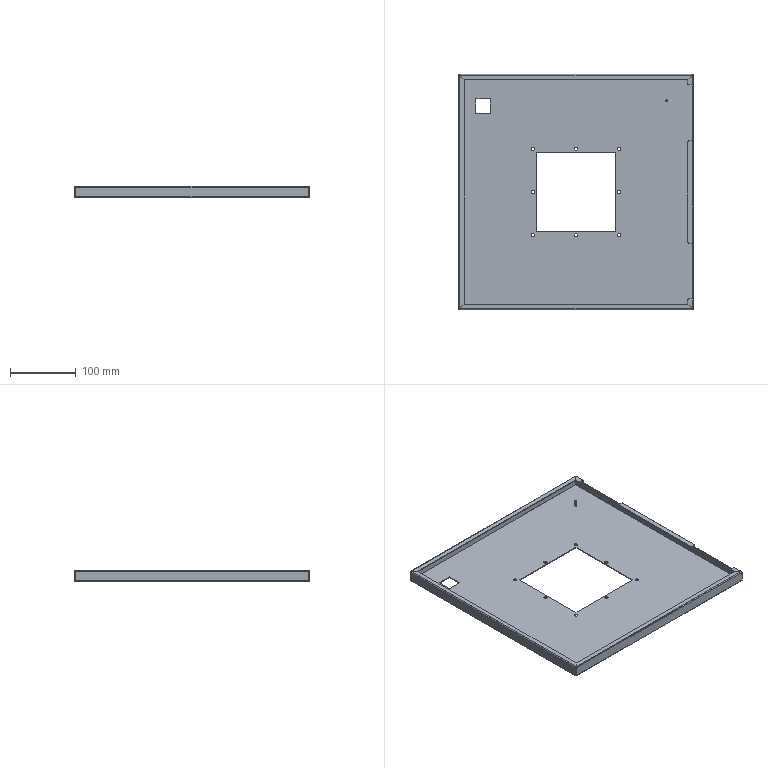Part | STEP file | Right door panel | 1 solid | 141 faces | box 356 x 357 x 17 mm | volume 169245 mm3 | plane 91 | cylinder 42 | spline 8 | commonest cylinder face diameters 5 x16 0.02 x10 2.42 x10 2 x4 3 x2